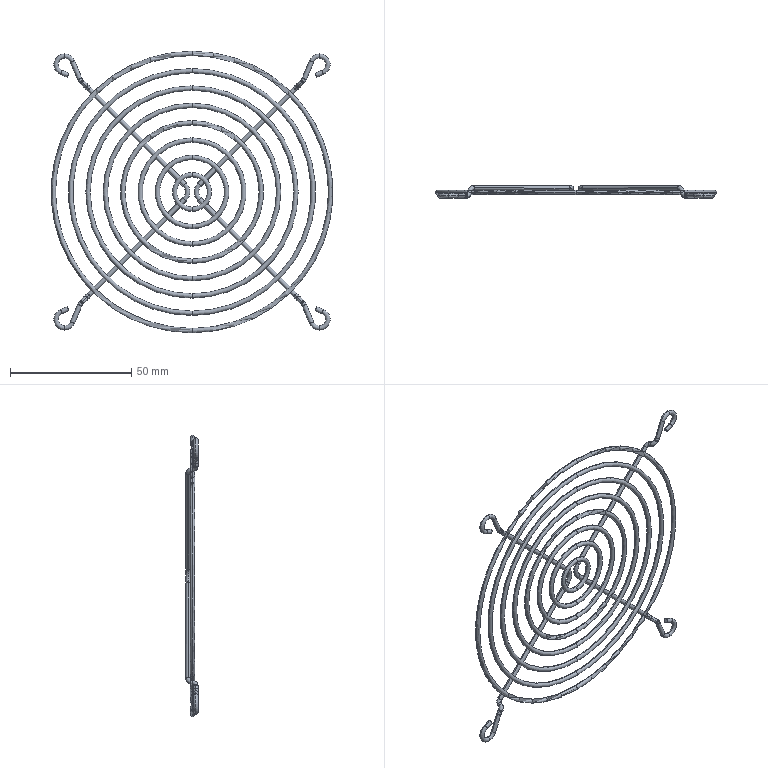Part | STEP file | FKL6622 cabinet fan and filter[FKL6622.230]_TX120 | 10 solids | 120 faces | box 116 x 5 x 116 mm | volume 5033 mm3 | torus 76 | cylinder 40 | plane 4 | commonest cylinder face diameters 1.8 x40